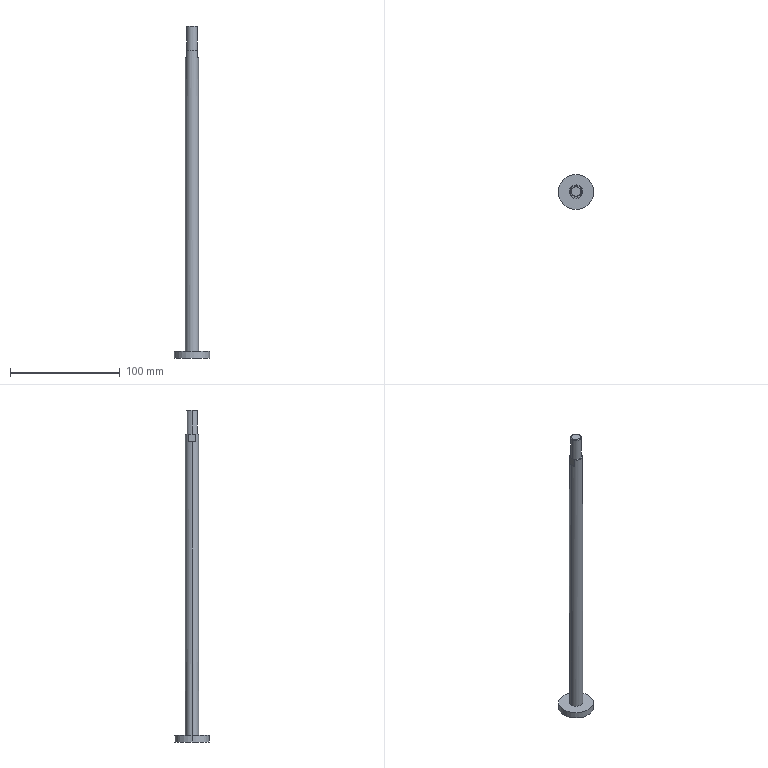Part | STEP file | 1 solid | 17 faces | box 32 x 32 x 303.2 mm | volume 37606 mm3 | plane 9 | cylinder 6 | cone 2 | commonest cylinder face diameters 10 x2 12 x2 32 x2
STEP:
#1=CARTESIAN_POINT('',(0.,0.,0.));
#2=DIRECTION('',(0.,0.,1.));
#3=DIRECTION('',(1.,0.,0.));
#4=AXIS2_PLACEMENT_3D('',#1,#2,#3);
#5=CARTESIAN_POINT('',(5.,0.,26.));
#6=VERTEX_POINT('',#5);
#7=CARTESIAN_POINT('',(-5.,0.,26.));
#8=VERTEX_POINT('',#7);
#9=CARTESIAN_POINT('',(0.,0.,26.));
#10=DIRECTION('',(0.,0.,1.));
#11=DIRECTION('',(1.,0.,0.));
#12=AXIS2_PLACEMENT_3D('',#9,#10,#11);
#13=CIRCLE('',#12,5.);
#14=CARTESIAN_POINT('',(0.,0.,26.));
#15=DIRECTION('',(0.,0.,1.));
#16=DIRECTION('',(1.,0.,0.));
#17=AXIS2_PLACEMENT_3D('',#14,#15,#16);
#18=CYLINDRICAL_SURFACE('',#17,5.);
#19=CARTESIAN_POINT('',(0.,0.));
#20=DIRECTION('',(1.,0.));
#21=VECTOR('',#20,1.);
#22=LINE('',#19,#21);
#23=(GEOMETRIC_REPRESENTATION_CONTEXT(2)PARAMETRIC_REPRESENTATION_CONTEXT()REPRESENTATION_CONTEXT('',''));
#24=DEFINITIONAL_REPRESENTATION('',(#22),#23);
#25=PCURVE('',#18,#24);
#26=CARTESIAN_POINT('',(0.,0.,26.));
#27=DIRECTION('',(0.,0.,-1.));
#28=DIRECTION('',(-1.,0.,0.));
#29=AXIS2_PLACEMENT_3D('',#26,#27,#28);
#30=PLANE('',#29);
#31=CARTESIAN_POINT('',(-5.,0.));
#32=CARTESIAN_POINT('',(-5.,8.66));
#33=CARTESIAN_POINT('',(2.5,4.33));
#34=CARTESIAN_POINT('',(10.,0.));
#35=CARTESIAN_POINT('',(2.5,-4.33));
#36=CARTESIAN_POINT('',(-5.,-8.66));
#37=CARTESIAN_POINT('',(-5.,0.));
#38=(BOUNDED_CURVE()B_SPLINE_CURVE(2,(#31,#32,#33,#34,#35,#36,#37),.UNSPECIFIED.,.T.,.F.)B_SPLINE_CURVE_WITH_KNOTS((1,2,2,2,2,1),(-2.094,0.,2.094,4.189,6.283,8.378),.UNSPECIFIED.)CURVE()GEOMETRIC_REPRESENTATION_ITEM()RATIONAL_B_SPLINE_CURVE((1.,0.5,1.,0.5,1.,0.5,1.))REPRESENTATION_ITEM(''));
#39=(GEOMETRIC_REPRESENTATION_CONTEXT(2)PARAMETRIC_REPRESENTATION_CONTEXT()REPRESENTATION_CONTEXT('',''));
#40=DEFINITIONAL_REPRESENTATION('',(#38),#39);
#41=PCURVE('',#30,#40);
#42=SURFACE_CURVE('',#13,(#25,#41),.PCURVE_S1.);
#43=EDGE_CURVE('',#6,#8,#42,.T.);
#44=ORIENTED_EDGE('',*,*,#43,.T.);
#45=CARTESIAN_POINT('',(-5.,0.,47.233));
#46=VERTEX_POINT('',#45);
#47=CARTESIAN_POINT('',(-5.,0.,26.));
#48=DIRECTION('',(0.,0.,1.));
#49=VECTOR('',#48,1.);
#50=LINE('',#47,#49);
#51=CARTESIAN_POINT('',(3.142,0.));
#52=DIRECTION('',(0.,1.));
#53=VECTOR('',#52,1.);
#54=LINE('',#51,#53);
#55=(GEOMETRIC_REPRESENTATION_CONTEXT(2)PARAMETRIC_REPRESENTATION_CONTEXT()REPRESENTATION_CONTEXT('',''));
#56=DEFINITIONAL_REPRESENTATION('',(#54),#55);
#57=PCURVE('',#18,#56);
#58=CARTESIAN_POINT('',(0.,0.,26.));
#59=DIRECTION('',(0.,0.,1.));
#60=DIRECTION('',(1.,0.,0.));
#61=AXIS2_PLACEMENT_3D('',#58,#59,#60);
#62=CYLINDRICAL_SURFACE('',#61,5.);
#63=CARTESIAN_POINT('',(3.142,0.));
#64=DIRECTION('',(0.,1.));
#65=VECTOR('',#64,1.);
#66=LINE('',#63,#65);
#67=(GEOMETRIC_REPRESENTATION_CONTEXT(2)PARAMETRIC_REPRESENTATION_CONTEXT()REPRESENTATION_CONTEXT('',''));
#68=DEFINITIONAL_REPRESENTATION('',(#66),#67);
#69=PCURVE('',#62,#68);
#70=SURFACE_CURVE('',#50,(#57,#69),.PCURVE_S1.);
#71=EDGE_CURVE('',#8,#46,#70,.T.);
#72=ORIENTED_EDGE('',*,*,#71,.T.);
#73=CARTESIAN_POINT('',(5.,0.,47.233));
#74=VERTEX_POINT('',#73);
#75=CARTESIAN_POINT('',(0.,0.,47.233));
#76=DIRECTION('',(0.,0.,1.));
#77=DIRECTION('',(1.,0.,0.));
#78=AXIS2_PLACEMENT_3D('',#75,#76,#77);
#79=CIRCLE('',#78,5.);
#80=CARTESIAN_POINT('',(0.,21.233));
#81=DIRECTION('',(1.,0.));
#82=VECTOR('',#81,1.);
#83=LINE('',#80,#82);
#84=(GEOMETRIC_REPRESENTATION_CONTEXT(2)PARAMETRIC_REPRESENTATION_CONTEXT()REPRESENTATION_CONTEXT('',''));
#85=DEFINITIONAL_REPRESENTATION('',(#83),#84);
#86=PCURVE('',#18,#85);
#87=CARTESIAN_POINT('',(0.,0.,47.233));
#88=DIRECTION('',(0.,0.,-1.));
#89=DIRECTION('',(-1.,0.,0.));
#90=AXIS2_PLACEMENT_3D('',#87,#88,#89);
#91=CONICAL_SURFACE('',#90,5.,0.7854);
#92=CARTESIAN_POINT('',(3.142,0.));
#93=DIRECTION('',(-1.,0.));
#94=VECTOR('',#93,1.);
#95=LINE('',#92,#94);
#96=(GEOMETRIC_REPRESENTATION_CONTEXT(2)PARAMETRIC_REPRESENTATION_CONTEXT()REPRESENTATION_CONTEXT('',''));
#97=DEFINITIONAL_REPRESENTATION('',(#95),#96);
#98=PCURVE('',#91,#97);
#99=SURFACE_CURVE('',#79,(#86,#98),.PCURVE_S1.);
#100=EDGE_CURVE('',#74,#46,#99,.T.);
#101=ORIENTED_EDGE('',*,*,#100,.F.);
#102=CARTESIAN_POINT('',(5.,0.,26.));
#103=DIRECTION('',(0.,0.,1.));
#104=VECTOR('',#103,1.);
#105=LINE('',#102,#104);
#106=CARTESIAN_POINT('',(0.,0.));
#107=DIRECTION('',(0.,1.));
#108=VECTOR('',#107,1.);
#109=LINE('',#106,#108);
#110=(GEOMETRIC_REPRESENTATION_CONTEXT(2)PARAMETRIC_REPRESENTATION_CONTEXT()REPRESENTATION_CONTEXT('',''));
#111=DEFINITIONAL_REPRESENTATION('',(#109),#110);
#112=PCURVE('',#18,#111);
#113=CARTESIAN_POINT('',(6.283,0.));
#114=DIRECTION('',(0.,1.));
#115=VECTOR('',#114,1.);
#116=LINE('',#113,#115);
#117=(GEOMETRIC_REPRESENTATION_CONTEXT(2)PARAMETRIC_REPRESENTATION_CONTEXT()REPRESENTATION_CONTEXT('',''));
#118=DEFINITIONAL_REPRESENTATION('',(#116),#117);
#119=PCURVE('',#62,#118);
#120=SURFACE_CURVE('',#105,(#112,#119),.PCURVE_S1.);
#121=EDGE_CURVE('',#6,#74,#120,.T.);
#122=ORIENTED_EDGE('',*,*,#121,.F.);
#123=EDGE_LOOP('',(#44,#72,#101,#122));
#124=FACE_BOUND('',#123,.T.);
#125=ADVANCED_FACE('',(#124),#18,.T.);
#126=CARTESIAN_POINT('',(4.233,0.,48.));
#127=VERTEX_POINT('',#126);
#128=CARTESIAN_POINT('',(-4.233,0.,48.));
#129=VERTEX_POINT('',#128);
#130=CARTESIAN_POINT('',(0.,0.,48.));
#131=DIRECTION('',(0.,0.,1.));
#132=DIRECTION('',(1.,0.,0.));
#133=AXIS2_PLACEMENT_3D('',#130,#131,#132);
#134=CIRCLE('',#133,4.233);
#135=CARTESIAN_POINT('',(3.142,-0.767));
#136=DIRECTION('',(-1.,0.));
#137=VECTOR('',#136,1.);
#138=LINE('',#135,#137);
#139=(GEOMETRIC_REPRESENTATION_CONTEXT(2)PARAMETRIC_REPRESENTATION_CONTEXT()REPRESENTATION_CONTEXT('',''));
#140=DEFINITIONAL_REPRESENTATION('',(#138),#139);
#141=PCURVE('',#91,#140);
#142=CARTESIAN_POINT('',(0.,0.,48.));
#143=DIRECTION('',(0.,0.,-1.));
#144=DIRECTION('',(-1.,0.,0.));
#145=AXIS2_PLACEMENT_3D('',#142,#143,#144);
#146=PLANE('',#145);
#147=CARTESIAN_POINT('',(-4.233,0.));
#148=CARTESIAN_POINT('',(-4.233,7.332));
#149=CARTESIAN_POINT('',(2.116,3.666));
#150=CARTESIAN_POINT('',(8.466,0.));
#151=CARTESIAN_POINT('',(2.116,-3.666));
#152=CARTESIAN_POINT('',(-4.233,-7.332));
#153=CARTESIAN_POINT('',(-4.233,0.));
#154=(BOUNDED_CURVE()B_SPLINE_CURVE(2,(#147,#148,#149,#150,#151,#152,#153),.UNSPECIFIED.,.T.,.F.)B_SPLINE_CURVE_WITH_KNOTS((1,2,2,2,2,1),(-2.094,0.,2.094,4.189,6.283,8.378),.UNSPECIFIED.)CURVE()GEOMETRIC_REPRESENTATION_ITEM()RATIONAL_B_SPLINE_CURVE((1.,0.5,1.,0.5,1.,0.5,1.))REPRESENTATION_ITEM(''));
#155=(GEOMETRIC_REPRESENTATION_CONTEXT(2)PARAMETRIC_REPRESENTATION_CONTEXT()REPRESENTATION_CONTEXT('',''));
#156=DEFINITIONAL_REPRESENTATION('',(#154),#155);
#157=PCURVE('',#146,#156);
#158=SURFACE_CURVE('',#134,(#141,#157),.PCURVE_S1.);
#159=EDGE_CURVE('',#127,#129,#158,.T.);
#160=ORIENTED_EDGE('',*,*,#159,.F.);
#161=CARTESIAN_POINT('',(5.,0.,47.233));
#162=DIRECTION('',(0.7071,0.,-0.7071));
#163=VECTOR('',#162,1.);
#164=LINE('',#161,#163);
#165=CARTESIAN_POINT('',(3.142,0.));
#166=DIRECTION('',(0.,1.));
#167=VECTOR('',#166,1.);
#168=LINE('',#165,#167);
#169=(GEOMETRIC_REPRESENTATION_CONTEXT(2)PARAMETRIC_REPRESENTATION_CONTEXT()REPRESENTATION_CONTEXT('',''));
#170=DEFINITIONAL_REPRESENTATION('',(#168),#169);
#171=PCURVE('',#91,#170);
#172=CARTESIAN_POINT('',(0.,0.,47.233));
#173=DIRECTION('',(0.,0.,-1.));
#174=DIRECTION('',(-1.,0.,0.));
#175=AXIS2_PLACEMENT_3D('',#172,#173,#174);
#176=CONICAL_SURFACE('',#175,5.,0.7854);
#177=CARTESIAN_POINT('',(3.142,0.));
#178=DIRECTION('',(0.,1.));
#179=VECTOR('',#178,1.);
#180=LINE('',#177,#179);
#181=(GEOMETRIC_REPRESENTATION_CONTEXT(2)PARAMETRIC_REPRESENTATION_CONTEXT()REPRESENTATION_CONTEXT('',''));
#182=DEFINITIONAL_REPRESENTATION('',(#180),#181);
#183=PCURVE('',#176,#182);
#184=SURFACE_CURVE('',#164,(#171,#183),.PCURVE_S1.);
#185=EDGE_CURVE('',#127,#74,#184,.T.);
#186=ORIENTED_EDGE('',*,*,#185,.T.);
#187=ORIENTED_EDGE('',*,*,#100,.T.);
#188=CARTESIAN_POINT('',(-5.,0.,47.233));
#189=DIRECTION('',(-0.7071,0.,-0.7071));
#190=VECTOR('',#189,1.);
#191=LINE('',#188,#190);
#192=CARTESIAN_POINT('',(0.,0.));
#193=DIRECTION('',(0.,1.));
#194=VECTOR('',#193,1.);
#195=LINE('',#192,#194);
#196=(GEOMETRIC_REPRESENTATION_CONTEXT(2)PARAMETRIC_REPRESENTATION_CONTEXT()REPRESENTATION_CONTEXT('',''));
#197=DEFINITIONAL_REPRESENTATION('',(#195),#196);
#198=PCURVE('',#91,#197);
#199=CARTESIAN_POINT('',(6.283,0.));
#200=DIRECTION('',(0.,1.));
#201=VECTOR('',#200,1.);
#202=LINE('',#199,#201);
#203=(GEOMETRIC_REPRESENTATION_CONTEXT(2)PARAMETRIC_REPRESENTATION_CONTEXT()REPRESENTATION_CONTEXT('',''));
#204=DEFINITIONAL_REPRESENTATION('',(#202),#203);
#205=PCURVE('',#176,#204);
#206=SURFACE_CURVE('',#191,(#198,#205),.PCURVE_S1.);
#207=EDGE_CURVE('',#129,#46,#206,.T.);
#208=ORIENTED_EDGE('',*,*,#207,.F.);
#209=EDGE_LOOP('',(#160,#186,#187,#208));
#210=FACE_BOUND('',#209,.T.);
#211=ADVANCED_FACE('',(#210),#91,.T.);
#212=CARTESIAN_POINT('',(16.,0.,-255.2));
#213=VERTEX_POINT('',#212);
#214=CARTESIAN_POINT('',(-16.,0.,-255.2));
#215=VERTEX_POINT('',#214);
#216=CARTESIAN_POINT('',(0.,0.,-255.2));
#217=DIRECTION('',(0.,0.,1.));
#218=DIRECTION('',(1.,0.,0.));
#219=AXIS2_PLACEMENT_3D('',#216,#217,#218);
#220=CIRCLE('',#219,16.);
#221=CARTESIAN_POINT('',(0.,0.,-255.2));
#222=DIRECTION('',(0.,0.,1.));
#223=DIRECTION('',(1.,0.,0.));
#224=AXIS2_PLACEMENT_3D('',#221,#222,#223);
#225=CYLINDRICAL_SURFACE('',#224,16.);
#226=CARTESIAN_POINT('',(0.,0.));
#227=DIRECTION('',(1.,0.));
#228=VECTOR('',#227,1.);
#229=LINE('',#226,#228);
#230=(GEOMETRIC_REPRESENTATION_CONTEXT(2)PARAMETRIC_REPRESENTATION_CONTEXT()REPRESENTATION_CONTEXT('',''));
#231=DEFINITIONAL_REPRESENTATION('',(#229),#230);
#232=PCURVE('',#225,#231);
#233=CARTESIAN_POINT('',(0.,16.,-255.2));
#234=DIRECTION('',(0.,0.,1.));
#235=DIRECTION('',(1.,0.,0.));
#236=AXIS2_PLACEMENT_3D('',#233,#234,#235);
#237=PLANE('',#236);
#238=CARTESIAN_POINT('',(0.,-16.));
#239=DIRECTION('',(1.,0.));
#240=AXIS2_PLACEMENT_2D('',#238,#239);
#241=CIRCLE('',#240,16.);
#242=(GEOMETRIC_REPRESENTATION_CONTEXT(2)PARAMETRIC_REPRESENTATION_CONTEXT()REPRESENTATION_CONTEXT('',''));
#243=DEFINITIONAL_REPRESENTATION('',(#241),#242);
#244=PCURVE('',#237,#243);
#245=SURFACE_CURVE('',#220,(#232,#244),.PCURVE_S1.);
#246=EDGE_CURVE('',#213,#215,#245,.T.);
#247=ORIENTED_EDGE('',*,*,#246,.T.);
#248=CARTESIAN_POINT('',(-16.,0.,-249.2));
#249=VERTEX_POINT('',#248);
#250=CARTESIAN_POINT('',(-16.,0.,-255.2));
#251=DIRECTION('',(0.,0.,1.));
#252=VECTOR('',#251,1.);
#253=LINE('',#250,#252);
#254=CARTESIAN_POINT('',(3.142,0.));
#255=DIRECTION('',(0.,1.));
#256=VECTOR('',#255,1.);
#257=LINE('',#254,#256);
#258=(GEOMETRIC_REPRESENTATION_CONTEXT(2)PARAMETRIC_REPRESENTATION_CONTEXT()REPRESENTATION_CONTEXT('',''));
#259=DEFINITIONAL_REPRESENTATION('',(#257),#258);
#260=PCURVE('',#225,#259);
#261=CARTESIAN_POINT('',(0.,0.,-255.2));
#262=DIRECTION('',(0.,0.,1.));
#263=DIRECTION('',(1.,0.,0.));
#264=AXIS2_PLACEMENT_3D('',#261,#262,#263);
#265=CYLINDRICAL_SURFACE('',#264,16.);
#266=CARTESIAN_POINT('',(3.142,0.));
#267=DIRECTION('',(0.,1.));
#268=VECTOR('',#267,1.);
#269=LINE('',#266,#268);
#270=(GEOMETRIC_REPRESENTATION_CONTEXT(2)PARAMETRIC_REPRESENTATION_CONTEXT()REPRESENTATION_CONTEXT('',''));
#271=DEFINITIONAL_REPRESENTATION('',(#269),#270);
#272=PCURVE('',#265,#271);
#273=SURFACE_CURVE('',#253,(#260,#272),.PCURVE_S1.);
#274=EDGE_CURVE('',#215,#249,#273,.T.);
#275=ORIENTED_EDGE('',*,*,#274,.T.);
#276=CARTESIAN_POINT('',(16.,0.,-249.2));
#277=VERTEX_POINT('',#276);
#278=CARTESIAN_POINT('',(0.,0.,-249.2));
#279=DIRECTION('',(0.,0.,1.));
#280=DIRECTION('',(1.,0.,0.));
#281=AXIS2_PLACEMENT_3D('',#278,#279,#280);
#282=CIRCLE('',#281,16.);
#283=CARTESIAN_POINT('',(0.,6.));
#284=DIRECTION('',(1.,0.));
#285=VECTOR('',#284,1.);
#286=LINE('',#283,#285);
#287=(GEOMETRIC_REPRESENTATION_CONTEXT(2)PARAMETRIC_REPRESENTATION_CONTEXT()REPRESENTATION_CONTEXT('',''));
#288=DEFINITIONAL_REPRESENTATION('',(#286),#287);
#289=PCURVE('',#225,#288);
#290=CARTESIAN_POINT('',(0.,6.,-249.2));
#291=DIRECTION('',(0.,0.,-1.));
#292=DIRECTION('',(-1.,0.,0.));
#293=AXIS2_PLACEMENT_3D('',#290,#291,#292);
#294=PLANE('',#293);
#295=CARTESIAN_POINT('',(-16.,-6.));
#296=CARTESIAN_POINT('',(-16.,21.713));
#297=CARTESIAN_POINT('',(8.,7.856));
#298=CARTESIAN_POINT('',(32.,-6.));
#299=CARTESIAN_POINT('',(8.,-19.856));
#300=CARTESIAN_POINT('',(-16.,-33.713));
#301=CARTESIAN_POINT('',(-16.,-6.));
#302=(BOUNDED_CURVE()B_SPLINE_CURVE(2,(#295,#296,#297,#298,#299,#300,#301),.UNSPECIFIED.,.T.,.F.)B_SPLINE_CURVE_WITH_KNOTS((1,2,2,2,2,1),(-2.094,0.,2.094,4.189,6.283,8.378),.UNSPECIFIED.)CURVE()GEOMETRIC_REPRESENTATION_ITEM()RATIONAL_B_SPLINE_CURVE((1.,0.5,1.,0.5,1.,0.5,1.))REPRESENTATION_ITEM(''));
#303=(GEOMETRIC_REPRESENTATION_CONTEXT(2)PARAMETRIC_REPRESENTATION_CONTEXT()REPRESENTATION_CONTEXT('',''));
#304=DEFINITIONAL_REPRESENTATION('',(#302),#303);
#305=PCURVE('',#294,#304);
#306=SURFACE_CURVE('',#282,(#289,#305),.PCURVE_S1.);
#307=EDGE_CURVE('',#277,#249,#306,.T.);
#308=ORIENTED_EDGE('',*,*,#307,.F.);
#309=CARTESIAN_POINT('',(16.,0.,-255.2));
#310=DIRECTION('',(0.,0.,1.));
#311=VECTOR('',#310,1.);
#312=LINE('',#309,#311);
#313=CARTESIAN_POINT('',(0.,0.));
#314=DIRECTION('',(0.,1.));
#315=VECTOR('',#314,1.);
#316=LINE('',#313,#315);
#317=(GEOMETRIC_REPRESENTATION_CONTEXT(2)PARAMETRIC_REPRESENTATION_CONTEXT()REPRESENTATION_CONTEXT('',''));
#318=DEFINITIONAL_REPRESENTATION('',(#316),#317);
#319=PCURVE('',#225,#318);
#320=CARTESIAN_POINT('',(6.283,0.));
#321=DIRECTION('',(0.,1.));
#322=VECTOR('',#321,1.);
#323=LINE('',#320,#322);
#324=(GEOMETRIC_REPRESENTATION_CONTEXT(2)PARAMETRIC_REPRESENTATION_CONTEXT()REPRESENTATION_CONTEXT('',''));
#325=DEFINITIONAL_REPRESENTATION('',(#323),#324);
#326=PCURVE('',#265,#325);
#327=SURFACE_CURVE('',#312,(#319,#326),.PCURVE_S1.);
#328=EDGE_CURVE('',#213,#277,#327,.T.);
#329=ORIENTED_EDGE('',*,*,#328,.F.);
#330=EDGE_LOOP('',(#247,#275,#308,#329));
#331=FACE_BOUND('',#330,.T.);
#332=ADVANCED_FACE('',(#331),#225,.T.);
#333=CARTESIAN_POINT('',(6.,0.,-249.2));
#334=VERTEX_POINT('',#333);
#335=CARTESIAN_POINT('',(-6.,0.,-249.2));
#336=VERTEX_POINT('',#335);
#337=CARTESIAN_POINT('',(0.,0.,-249.2));
#338=DIRECTION('',(0.,0.,1.));
#339=DIRECTION('',(1.,0.,0.));
#340=AXIS2_PLACEMENT_3D('',#337,#338,#339);
#341=CIRCLE('',#340,6.);
#342=CARTESIAN_POINT('',(0.,0.,-255.2));
#343=DIRECTION('',(0.,0.,1.));
#344=DIRECTION('',(1.,0.,0.));
#345=AXIS2_PLACEMENT_3D('',#342,#343,#344);
#346=CYLINDRICAL_SURFACE('',#345,6.);
#347=CARTESIAN_POINT('',(0.,6.));
#348=DIRECTION('',(1.,0.));
#349=VECTOR('',#348,1.);
#350=LINE('',#347,#349);
#351=(GEOMETRIC_REPRESENTATION_CONTEXT(2)PARAMETRIC_REPRESENTATION_CONTEXT()REPRESENTATION_CONTEXT('',''));
#352=DEFINITIONAL_REPRESENTATION('',(#350),#351);
#353=PCURVE('',#346,#352);
#354=CARTESIAN_POINT('',(-6.,-6.));
#355=CARTESIAN_POINT('',(-6.,4.392));
#356=CARTESIAN_POINT('',(3.,-0.8038));
#357=CARTESIAN_POINT('',(12.,-6.));
#358=CARTESIAN_POINT('',(3.,-11.196));
#359=CARTESIAN_POINT('',(-6.,-16.392));
#360=CARTESIAN_POINT('',(-6.,-6.));
#361=(BOUNDED_CURVE()B_SPLINE_CURVE(2,(#354,#355,#356,#357,#358,#359,#360),.UNSPECIFIED.,.T.,.F.)B_SPLINE_CURVE_WITH_KNOTS((1,2,2,2,2,1),(-2.094,0.,2.094,4.189,6.283,8.378),.UNSPECIFIED.)CURVE()GEOMETRIC_REPRESENTATION_ITEM()RATIONAL_B_SPLINE_CURVE((1.,0.5,1.,0.5,1.,0.5,1.))REPRESENTATION_ITEM(''));
#362=(GEOMETRIC_REPRESENTATION_CONTEXT(2)PARAMETRIC_REPRESENTATION_CONTEXT()REPRESENTATION_CONTEXT('',''));
#363=DEFINITIONAL_REPRESENTATION('',(#361),#362);
#364=PCURVE('',#294,#363);
#365=SURFACE_CURVE('',#341,(#353,#364),.PCURVE_S1.);
#366=EDGE_CURVE('',#334,#336,#365,.T.);
#367=ORIENTED_EDGE('',*,*,#366,.T.);
#368=CARTESIAN_POINT('',(-6.,0.,19.));
#369=VERTEX_POINT('',#368);
#370=CARTESIAN_POINT('',(-6.,0.,-255.2));
#371=DIRECTION('',(0.,0.,1.));
#372=VECTOR('',#371,1.);
#373=LINE('',#370,#372);
#374=CARTESIAN_POINT('',(3.142,0.));
#375=DIRECTION('',(0.,1.));
#376=VECTOR('',#375,1.);
#377=LINE('',#374,#376);
#378=(GEOMETRIC_REPRESENTATION_CONTEXT(2)PARAMETRIC_REPRESENTATION_CONTEXT()REPRESENTATION_CONTEXT('',''));
#379=DEFINITIONAL_REPRESENTATION('',(#377),#378);
#380=PCURVE('',#346,#379);
#381=CARTESIAN_POINT('',(0.,0.,-255.2));
#382=DIRECTION('',(0.,0.,1.));
#383=DIRECTION('',(1.,0.,0.));
#384=AXIS2_PLACEMENT_3D('',#381,#382,#383);
#385=CYLINDRICAL_SURFACE('',#384,6.);
#386=CARTESIAN_POINT('',(3.142,0.));
#387=DIRECTION('',(0.,1.));
#388=VECTOR('',#387,1.);
#389=LINE('',#386,#388);
#390=(GEOMETRIC_REPRESENTATION_CONTEXT(2)PARAMETRIC_REPRESENTATION_CONTEXT()REPRESENTATION_CONTEXT('',''));
#391=DEFINITIONAL_REPRESENTATION('',(#389),#390);
#392=PCURVE('',#385,#391);
#393=SURFACE_CURVE('',#373,(#380,#392),.PCURVE_S1.);
#394=EDGE_CURVE('',#336,#369,#393,.T.);
#395=ORIENTED_EDGE('',*,*,#394,.T.);
#396=CARTESIAN_POINT('',(-5.,3.317,19.));
#397=VERTEX_POINT('',#396);
#398=CARTESIAN_POINT('',(0.,0.,19.));
#399=DIRECTION('',(0.,0.,1.));
#400=DIRECTION('',(1.,0.,0.));
#401=AXIS2_PLACEMENT_3D('',#398,#399,#400);
#402=CIRCLE('',#401,6.);
#403=CARTESIAN_POINT('',(0.,274.2));
#404=DIRECTION('',(1.,0.));
#405=VECTOR('',#404,1.);
#406=LINE('',#403,#405);
#407=(GEOMETRIC_REPRESENTATION_CONTEXT(2)PARAMETRIC_REPRESENTATION_CONTEXT()REPRESENTATION_CONTEXT('',''));
#408=DEFINITIONAL_REPRESENTATION('',(#406),#407);
#409=PCURVE('',#346,#408);
#410=CARTESIAN_POINT('',(0.,0.,19.));
#411=DIRECTION('',(0.,0.,1.));
#412=DIRECTION('',(1.,0.,0.));
#413=AXIS2_PLACEMENT_3D('',#410,#411,#412);
#414=PLANE('',#413);
#415=CARTESIAN_POINT('',(0.,0.));
#416=DIRECTION('',(1.,0.));
#417=AXIS2_PLACEMENT_2D('',#415,#416);
#418=CIRCLE('',#417,6.);
#419=(GEOMETRIC_REPRESENTATION_CONTEXT(2)PARAMETRIC_REPRESENTATION_CONTEXT()REPRESENTATION_CONTEXT('',''));
#420=DEFINITIONAL_REPRESENTATION('',(#418),#419);
#421=PCURVE('',#414,#420);
#422=SURFACE_CURVE('',#402,(#409,#421),.PCURVE_S1.);
#423=EDGE_CURVE('',#397,#369,#422,.T.);
#424=ORIENTED_EDGE('',*,*,#423,.F.);
#425=CARTESIAN_POINT('',(-5.,3.317,26.));
#426=VERTEX_POINT('',#425);
#427=CARTESIAN_POINT('',(-5.,3.317,-255.2));
#428=DIRECTION('',(0.,0.,1.));
#429=VECTOR('',#428,1.);
#430=LINE('',#427,#429);
#431=CARTESIAN_POINT('',(2.556,0.));
#432=DIRECTION('',(0.,1.));
#433=VECTOR('',#432,1.);
#434=LINE('',#431,#433);
#435=(GEOMETRIC_REPRESENTATION_CONTEXT(2)PARAMETRIC_REPRESENTATION_CONTEXT()REPRESENTATION_CONTEXT('',''));
#436=DEFINITIONAL_REPRESENTATION('',(#434),#435);
#437=PCURVE('',#346,#436);
#438=CARTESIAN_POINT('',(-5.,-10.,19.));
#439=DIRECTION('',(1.,0.,0.));
#440=DIRECTION('',(0.,0.,-1.));
#441=AXIS2_PLACEMENT_3D('',#438,#439,#440);
#442=PLANE('',#441);
#443=CARTESIAN_POINT('',(274.2,13.317));
#444=DIRECTION('',(-1.,0.));
#445=VECTOR('',#444,1.);
#446=LINE('',#443,#445);
#447=(GEOMETRIC_REPRESENTATION_CONTEXT(2)PARAMETRIC_REPRESENTATION_CONTEXT()REPRESENTATION_CONTEXT('',''));
#448=DEFINITIONAL_REPRESENTATION('',(#446),#447);
#449=PCURVE('',#442,#448);
#450=SURFACE_CURVE('',#430,(#437,#449),.PCURVE_S1.);
#451=EDGE_CURVE('',#397,#426,#450,.T.);
#452=ORIENTED_EDGE('',*,*,#451,.T.);
#453=CARTESIAN_POINT('',(5.,3.317,26.));
#454=VERTEX_POINT('',#453);
#455=CARTESIAN_POINT('',(0.,0.,26.));
#456=DIRECTION('',(0.,0.,1.));
#457=DIRECTION('',(1.,0.,0.));
#458=AXIS2_PLACEMENT_3D('',#455,#456,#457);
#459=CIRCLE('',#458,6.);
#460=CARTESIAN_POINT('',(0.,281.2));
#461=DIRECTION('',(1.,0.));
#462=VECTOR('',#461,1.);
#463=LINE('',#460,#462);
#464=(GEOMETRIC_REPRESENTATION_CONTEXT(2)PARAMETRIC_REPRESENTATION_CONTEXT()REPRESENTATION_CONTEXT('',''));
#465=DEFINITIONAL_REPRESENTATION('',(#463),#464);
#466=PCURVE('',#346,#465);
#467=CARTESIAN_POINT('',(-6.,0.));
#468=CARTESIAN_POINT('',(-6.,10.392));
#469=CARTESIAN_POINT('',(3.,5.196));
#470=CARTESIAN_POINT('',(12.,0.));
#471=CARTESIAN_POINT('',(3.,-5.196));
#472=CARTESIAN_POINT('',(-6.,-10.392));
#473=CARTESIAN_POINT('',(-6.,0.));
#474=(BOUNDED_CURVE()B_SPLINE_CURVE(2,(#467,#468,#469,#470,#471,#472,#473),.UNSPECIFIED.,.T.,.F.)B_SPLINE_CURVE_WITH_KNOTS((1,2,2,2,2,1),(-2.094,0.,2.094,4.189,6.283,8.378),.UNSPECIFIED.)CURVE()GEOMETRIC_REPRESENTATION_ITEM()RATIONAL_B_SPLINE_CURVE((1.,0.5,1.,0.5,1.,0.5,1.))REPRESENTATION_ITEM(''));
#475=(GEOMETRIC_REPRESENTATION_CONTEXT(2)PARAMETRIC_REPRESENTATION_CONTEXT()REPRESENTATION_CONTEXT('',''));
#476=DEFINITIONAL_REPRESENTATION('',(#474),#475);
#477=PCURVE('',#30,#476);
#478=SURFACE_CURVE('',#459,(#466,#477),.PCURVE_S1.);
#479=EDGE_CURVE('',#454,#426,#478,.T.);
#480=ORIENTED_EDGE('',*,*,#479,.F.);
#481=CARTESIAN_POINT('',(5.,3.317,19.));
#482=VERTEX_POINT('',#481);
#483=CARTESIAN_POINT('',(5.,3.317,-255.2));
#484=DIRECTION('',(0.,0.,-1.));
#485=VECTOR('',#484,1.);
#486=LINE('',#483,#485);
#487=CARTESIAN_POINT('',(0.5857,0.));
#488=DIRECTION('',(0.,-1.));
#489=VECTOR('',#488,1.);
#490=LINE('',#487,#489);
#491=(GEOMETRIC_REPRESENTATION_CONTEXT(2)PARAMETRIC_REPRESENTATION_CONTEXT()REPRESENTATION_CONTEXT('',''));
#492=DEFINITIONAL_REPRESENTATION('',(#490),#491);
#493=PCURVE('',#346,#492);
#494=CARTESIAN_POINT('',(5.,10.,19.));
#495=DIRECTION('',(-1.,0.,0.));
#496=DIRECTION('',(0.,0.,1.));
#497=AXIS2_PLACEMENT_3D('',#494,#495,#496);
#498=PLANE('',#497);
#499=CARTESIAN_POINT('',(-274.2,-6.683));
#500=DIRECTION('',(-1.,0.));
#501=VECTOR('',#500,1.);
#502=LINE('',#499,#501);
#503=(GEOMETRIC_REPRESENTATION_CONTEXT(2)PARAMETRIC_REPRESENTATION_CONTEXT()REPRESENTATION_CONTEXT('',''));
#504=DEFINITIONAL_REPRESENTATION('',(#502),#503);
#505=PCURVE('',#498,#504);
#506=SURFACE_CURVE('',#486,(#493,#505),.PCURVE_S1.);
#507=EDGE_CURVE('',#454,#482,#506,.T.);
#508=ORIENTED_EDGE('',*,*,#507,.T.);
#509=CARTESIAN_POINT('',(6.,0.,19.));
#510=VERTEX_POINT('',#509);
#511=CARTESIAN_POINT('',(0.,0.,19.));
#512=DIRECTION('',(0.,0.,1.));
#513=DIRECTION('',(1.,0.,0.));
#514=AXIS2_PLACEMENT_3D('',#511,#512,#513);
#515=CIRCLE('',#514,6.);
#516=CARTESIAN_POINT('',(0.,274.2));
#517=DIRECTION('',(1.,0.));
#518=VECTOR('',#517,1.);
#519=LINE('',#516,#518);
#520=(GEOMETRIC_REPRESENTATION_CONTEXT(2)PARAMETRIC_REPRESENTATION_CONTEXT()REPRESENTATION_CONTEXT('',''));
#521=DEFINITIONAL_REPRESENTATION('',(#519),#520);
#522=PCURVE('',#346,#521);
#523=CARTESIAN_POINT('',(0.,0.,19.));
#524=DIRECTION('',(0.,0.,1.));
#525=DIRECTION('',(1.,0.,0.));
#526=AXIS2_PLACEMENT_3D('',#523,#524,#525);
#527=PLANE('',#526);
#528=CARTESIAN_POINT('',(0.,0.));
#529=DIRECTION('',(1.,0.));
#530=AXIS2_PLACEMENT_2D('',#528,#529);
#531=CIRCLE('',#530,6.);
#532=(GEOMETRIC_REPRESENTATION_CONTEXT(2)PARAMETRIC_REPRESENTATION_CONTEXT()REPRESENTATION_CONTEXT('',''));
#533=DEFINITIONAL_REPRESENTATION('',(#531),#532);
#534=PCURVE('',#527,#533);
#535=SURFACE_CURVE('',#515,(#522,#534),.PCURVE_S1.);
#536=EDGE_CURVE('',#510,#482,#535,.T.);
#537=ORIENTED_EDGE('',*,*,#536,.F.);
#538=CARTESIAN_POINT('',(6.,0.,-255.2));
#539=DIRECTION('',(0.,0.,1.));
#540=VECTOR('',#539,1.);
#541=LINE('',#538,#540);
#542=CARTESIAN_POINT('',(0.,0.));
#543=DIRECTION('',(0.,1.));
#544=VECTOR('',#543,1.);
#545=LINE('',#542,#544);
#546=(GEOMETRIC_REPRESENTATION_CONTEXT(2)PARAMETRIC_REPRESENTATION_CONTEXT()REPRESENTATION_CONTEXT('',''));
#547=DEFINITIONAL_REPRESENTATION('',(#545),#546);
#548=PCURVE('',#346,#547);
#549=CARTESIAN_POINT('',(6.283,0.));
#550=DIRECTION('',(0.,1.));
#551=VECTOR('',#550,1.);
#552=LINE('',#549,#551);
#553=(GEOMETRIC_REPRESENTATION_CONTEXT(2)PARAMETRIC_REPRESENTATION_CONTEXT()REPRESENTATION_CONTEXT('',''));
#554=DEFINITIONAL_REPRESENTATION('',(#552),#553);
#555=PCURVE('',#385,#554);
#556=SURFACE_CURVE('',#541,(#548,#555),.PCURVE_S1.);
#557=EDGE_CURVE('',#334,#510,#556,.T.);
#558=ORIENTED_EDGE('',*,*,#557,.F.);
#559=EDGE_LOOP('',(#367,#395,#424,#452,#480,#508,#537,#558));
#560=FACE_BOUND('',#559,.T.);
#561=ADVANCED_FACE('',(#560),#346,.T.);
#562=ORIENTED_EDGE('',*,*,#43,.F.);
#563=CARTESIAN_POINT('',(5.,10.,26.));
#564=DIRECTION('',(0.,-1.,0.));
#565=VECTOR('',#564,1.);
#566=LINE('',#563,#565);
#567=CARTESIAN_POINT('',(-5.,10.));
#568=DIRECTION('',(0.,-1.));
#569=VECTOR('',#568,1.);
#570=LINE('',#567,#569);
#571=(GEOMETRIC_REPRESENTATION_CONTEXT(2)PARAMETRIC_REPRESENTATION_CONTEXT()REPRESENTATION_CONTEXT('',''));
#572=DEFINITIONAL_REPRESENTATION('',(#570),#571);
#573=PCURVE('',#30,#572);
#574=CARTESIAN_POINT('',(7.,0.));
#575=DIRECTION('',(0.,-1.));
#576=VECTOR('',#575,1.);
#577=LINE('',#574,#576);
#578=(GEOMETRIC_REPRESENTATION_CONTEXT(2)PARAMETRIC_REPRESENTATION_CONTEXT()REPRESENTATION_CONTEXT('',''));
#579=DEFINITIONAL_REPRESENTATION('',(#577),#578);
#580=PCURVE('',#498,#579);
#581=SURFACE_CURVE('',#566,(#573,#580),.PCURVE_S1.);
#582=EDGE_CURVE('',#454,#6,#581,.T.);
#583=ORIENTED_EDGE('',*,*,#582,.F.);
#584=ORIENTED_EDGE('',*,*,#479,.T.);
#585=CARTESIAN_POINT('',(-5.,-10.,26.));
#586=DIRECTION('',(0.,1.,0.));
#587=VECTOR('',#586,1.);
#588=LINE('',#585,#587);
#589=CARTESIAN_POINT('',(5.,-10.));
#590=DIRECTION('',(0.,1.));
#591=VECTOR('',#590,1.);
#592=LINE('',#589,#591);
#593=(GEOMETRIC_REPRESENTATION_CONTEXT(2)PARAMETRIC_REPRESENTATION_CONTEXT()REPRESENTATION_CONTEXT('',''));
#594=DEFINITIONAL_REPRESENTATION('',(#592),#593);
#595=PCURVE('',#30,#594);
#596=CARTESIAN_POINT('',(-7.,0.));
#597=DIRECTION('',(0.,1.));
#598=VECTOR('',#597,1.);
#599=LINE('',#596,#598);
#600=(GEOMETRIC_REPRESENTATION_CONTEXT(2)PARAMETRIC_REPRESENTATION_CONTEXT()REPRESENTATION_CONTEXT('',''));
#601=DEFINITIONAL_REPRESENTATION('',(#599),#600);
#602=PCURVE('',#442,#601);
#603=SURFACE_CURVE('',#588,(#595,#602),.PCURVE_S1.);
#604=EDGE_CURVE('',#8,#426,#603,.T.);
#605=ORIENTED_EDGE('',*,*,#604,.F.);
#606=EDGE_LOOP('',(#562,#583,#584,#605));
#607=FACE_BOUND('',#606,.T.);
#608=ADVANCED_FACE('',(#607),#30,.F.);
#609=CARTESIAN_POINT('',(0.,0.,26.));
#610=DIRECTION('',(0.,0.,1.));
#611=DIRECTION('',(1.,0.,0.));
#612=AXIS2_PLACEMENT_3D('',#609,#610,#611);
#613=CIRCLE('',#612,5.);
#614=CARTESIAN_POINT('',(0.,0.,26.));
#615=DIRECTION('',(0.,0.,-1.));
#616=DIRECTION('',(-1.,0.,0.));
#617=AXIS2_PLACEMENT_3D('',#614,#615,#616);
#618=PLANE('',#617);
#619=CARTESIAN_POINT('',(-5.,0.));
#620=CARTESIAN_POINT('',(-5.,8.66));
#621=CARTESIAN_POINT('',(2.5,4.33));
#622=CARTESIAN_POINT('',(10.,0.));
#623=CARTESIAN_POINT('',(2.5,-4.33));
#624=CARTESIAN_POINT('',(-5.,-8.66));
#625=CARTESIAN_POINT('',(-5.,0.));
#626=(BOUNDED_CURVE()B_SPLINE_CURVE(2,(#619,#620,#621,#622,#623,#624,#625),.UNSPECIFIED.,.T.,.F.)B_SPLINE_CURVE_WITH_KNOTS((1,2,2,2,2,1),(-2.094,0.,2.094,4.189,6.283,8.378),.UNSPECIFIED.)CURVE()GEOMETRIC_REPRESENTATION_ITEM()RATIONAL_B_SPLINE_CURVE((1.,0.5,1.,0.5,1.,0.5,1.))REPRESENTATION_ITEM(''));
#627=(GEOMETRIC_REPRESENTATION_CONTEXT(2)PARAMETRIC_REPRESENTATION_CONTEXT()REPRESENTATION_CONTEXT('',''));
#628=DEFINITIONAL_REPRESENTATION('',(#626),#627);
#629=PCURVE('',#618,#628);
#630=CARTESIAN_POINT('',(0.,0.));
#631=DIRECTION('',(1.,0.));
#632=VECTOR('',#631,1.);
#633=LINE('',#630,#632);
#634=(GEOMETRIC_REPRESENTATION_CONTEXT(2)PARAMETRIC_REPRESENTATION_CONTEXT()REPRESENTATION_CONTEXT('',''));
#635=DEFINITIONAL_REPRESENTATION('',(#633),#634);
#636=PCURVE('',#62,#635);
#637=SURFACE_CURVE('',#613,(#629,#636),.PCURVE_S1.);
#638=EDGE_CURVE('',#8,#6,#637,.T.);
#639=ORIENTED_EDGE('',*,*,#638,.F.);
#640=CARTESIAN_POINT('',(-5.,-3.317,26.));
#641=VERTEX_POINT('',#640);
#642=CARTESIAN_POINT('',(-5.,-10.,26.));
#643=DIRECTION('',(0.,1.,0.));
#644=VECTOR('',#643,1.);
#645=LINE('',#642,#644);
#646=CARTESIAN_POINT('',(5.,-10.));
#647=DIRECTION('',(0.,1.));
#648=VECTOR('',#647,1.);
#649=LINE('',#646,#648);
#650=(GEOMETRIC_REPRESENTATION_CONTEXT(2)PARAMETRIC_REPRESENTATION_CONTEXT()REPRESENTATION_CONTEXT('',''));
#651=DEFINITIONAL_REPRESENTATION('',(#649),#650);
#652=PCURVE('',#618,#651);
#653=CARTESIAN_POINT('',(-7.,0.));
#654=DIRECTION('',(0.,1.));
#655=VECTOR('',#654,1.);
#656=LINE('',#653,#655);
#657=(GEOMETRIC_REPRESENTATION_CONTEXT(2)PARAMETRIC_REPRESENTATION_CONTEXT()REPRESENTATION_CONTEXT('',''));
#658=DEFINITIONAL_REPRESENTATION('',(#656),#657);
#659=PCURVE('',#442,#658);
#660=SURFACE_CURVE('',#645,(#652,#659),.PCURVE_S1.);
#661=EDGE_CURVE('',#641,#8,#660,.T.);
#662=ORIENTED_EDGE('',*,*,#661,.F.);
#663=CARTESIAN_POINT('',(5.,-3.317,26.));
#664=VERTEX_POINT('',#663);
#665=CARTESIAN_POINT('',(0.,0.,26.));
#666=DIRECTION('',(0.,0.,1.));
#667=DIRECTION('',(1.,0.,0.));
#668=AXIS2_PLACEMENT_3D('',#665,#666,#667);
#669=CIRCLE('',#668,6.);
#670=CARTESIAN_POINT('',(-6.,0.));
#671=CARTESIAN_POINT('',(-6.,10.392));
#672=CARTESIAN_POINT('',(3.,5.196));
#673=CARTESIAN_POINT('',(12.,0.));
#674=CARTESIAN_POINT('',(3.,-5.196));
#675=CARTESIAN_POINT('',(-6.,-10.392));
#676=CARTESIAN_POINT('',(-6.,0.));
#677=(BOUNDED_CURVE()B_SPLINE_CURVE(2,(#670,#671,#672,#673,#674,#675,#676),.UNSPECIFIED.,.T.,.F.)B_SPLINE_CURVE_WITH_KNOTS((1,2,2,2,2,1),(-2.094,0.,2.094,4.189,6.283,8.378),.UNSPECIFIED.)CURVE()GEOMETRIC_REPRESENTATION_ITEM()RATIONAL_B_SPLINE_CURVE((1.,0.5,1.,0.5,1.,0.5,1.))REPRESENTATION_ITEM(''));
#678=(GEOMETRIC_REPRESENTATION_CONTEXT(2)PARAMETRIC_REPRESENTATION_CONTEXT()REPRESENTATION_CONTEXT('',''));
#679=DEFINITIONAL_REPRESENTATION('',(#677),#678);
#680=PCURVE('',#618,#679);
#681=CARTESIAN_POINT('',(0.,281.2));
#682=DIRECTION('',(1.,0.));
#683=VECTOR('',#682,1.);
#684=LINE('',#681,#683);
#685=(GEOMETRIC_REPRESENTATION_CONTEXT(2)PARAMETRIC_REPRESENTATION_CONTEXT()REPRESENTATION_CONTEXT('',''));
#686=DEFINITIONAL_REPRESENTATION('',(#684),#685);
#687=PCURVE('',#385,#686);
#688=SURFACE_CURVE('',#669,(#680,#687),.PCURVE_S1.);
#689=EDGE_CURVE('',#641,#664,#688,.T.);
#690=ORIENTED_EDGE('',*,*,#689,.T.);
#691=CARTESIAN_POINT('',(5.,10.,26.));
#692=DIRECTION('',(0.,-1.,0.));
#693=VECTOR('',#692,1.);
#694=LINE('',#691,#693);
#695=CARTESIAN_POINT('',(-5.,10.));
#696=DIRECTION('',(0.,-1.));
#697=VECTOR('',#696,1.);
#698=LINE('',#695,#697);
#699=(GEOMETRIC_REPRESENTATION_CONTEXT(2)PARAMETRIC_REPRESENTATION_CONTEXT()REPRESENTATION_CONTEXT('',''));
#700=DEFINITIONAL_REPRESENTATION('',(#698),#699);
#701=PCURVE('',#618,#700);
#702=CARTESIAN_POINT('',(7.,0.));
#703=DIRECTION('',(0.,-1.));
#704=VECTOR('',#703,1.);
#705=LINE('',#702,#704);
#706=(GEOMETRIC_REPRESENTATION_CONTEXT(2)PARAMETRIC_REPRESENTATION_CONTEXT()REPRESENTATION_CONTEXT('',''));
#707=DEFINITIONAL_REPRESENTATION('',(#705),#706);
#708=PCURVE('',#498,#707);
#709=SURFACE_CURVE('',#694,(#701,#708),.PCURVE_S1.);
#710=EDGE_CURVE('',#6,#664,#709,.T.);
#711=ORIENTED_EDGE('',*,*,#710,.F.);
#712=EDGE_LOOP('',(#639,#662,#690,#711));
#713=FACE_BOUND('',#712,.T.);
#714=ADVANCED_FACE('',(#713),#618,.F.);
#715=ORIENTED_EDGE('',*,*,#394,.F.);
#716=CARTESIAN_POINT('',(0.,0.,-249.2));
#717=DIRECTION('',(0.,0.,1.));
#718=DIRECTION('',(1.,0.,0.));
#719=AXIS2_PLACEMENT_3D('',#716,#717,#718);
#720=CIRCLE('',#719,6.);
#721=CARTESIAN_POINT('',(0.,6.));
#722=DIRECTION('',(1.,0.));
#723=VECTOR('',#722,1.);
#724=LINE('',#721,#723);
#725=(GEOMETRIC_REPRESENTATION_CONTEXT(2)PARAMETRIC_REPRESENTATION_CONTEXT()REPRESENTATION_CONTEXT('',''));
#726=DEFINITIONAL_REPRESENTATION('',(#724),#725);
#727=PCURVE('',#385,#726);
#728=CARTESIAN_POINT('',(-6.,-6.));
#729=CARTESIAN_POINT('',(-6.,4.392));
#730=CARTESIAN_POINT('',(3.,-0.8038));
#731=CARTESIAN_POINT('',(12.,-6.));
#732=CARTESIAN_POINT('',(3.,-11.196));
#733=CARTESIAN_POINT('',(-6.,-16.392));
#734=CARTESIAN_POINT('',(-6.,-6.));
#735=(BOUNDED_CURVE()B_SPLINE_CURVE(2,(#728,#729,#730,#731,#732,#733,#734),.UNSPECIFIED.,.T.,.F.)B_SPLINE_CURVE_WITH_KNOTS((1,2,2,2,2,1),(-2.094,0.,2.094,4.189,6.283,8.378),.UNSPECIFIED.)CURVE()GEOMETRIC_REPRESENTATION_ITEM()RATIONAL_B_SPLINE_CURVE((1.,0.5,1.,0.5,1.,0.5,1.))REPRESENTATION_ITEM(''));
#736=(GEOMETRIC_REPRESENTATION_CONTEXT(2)PARAMETRIC_REPRESENTATION_CONTEXT()REPRESENTATION_CONTEXT('',''));
#737=DEFINITIONAL_REPRESENTATION('',(#735),#736);
#738=PCURVE('',#294,#737);
#739=SURFACE_CURVE('',#720,(#727,#738),.PCURVE_S1.);
#740=EDGE_CURVE('',#336,#334,#739,.T.);
#741=ORIENTED_EDGE('',*,*,#740,.T.);
#742=ORIENTED_EDGE('',*,*,#557,.T.);
#743=CARTESIAN_POINT('',(5.,-3.317,19.));
#744=VERTEX_POINT('',#743);
#745=CARTESIAN_POINT('',(0.,0.,19.));
#746=DIRECTION('',(0.,0.,1.));
#747=DIRECTION('',(1.,0.,0.));
#748=AXIS2_PLACEMENT_3D('',#745,#746,#747);
#749=CIRCLE('',#748,6.);
#750=CARTESIAN_POINT('',(0.,274.2));
#751=DIRECTION('',(1.,0.));
#752=VECTOR('',#751,1.);
#753=LINE('',#750,#752);
#754=(GEOMETRIC_REPRESENTATION_CONTEXT(2)PARAMETRIC_REPRESENTATION_CONTEXT()REPRESENTATION_CONTEXT('',''));
#755=DEFINITIONAL_REPRESENTATION('',(#753),#754);
#756=PCURVE('',#385,#755);
#757=CARTESIAN_POINT('',(0.,0.));
#758=DIRECTION('',(1.,0.));
#759=AXIS2_PLACEMENT_2D('',#757,#758);
#760=CIRCLE('',#759,6.);
#761=(GEOMETRIC_REPRESENTATION_CONTEXT(2)PARAMETRIC_REPRESENTATION_CONTEXT()REPRESENTATION_CONTEXT('',''));
#762=DEFINITIONAL_REPRESENTATION('',(#760),#761);
#763=PCURVE('',#527,#762);
#764=SURFACE_CURVE('',#749,(#756,#763),.PCURVE_S1.);
#765=EDGE_CURVE('',#744,#510,#764,.T.);
#766=ORIENTED_EDGE('',*,*,#765,.F.);
#767=CARTESIAN_POINT('',(5.,-3.317,-255.2));
#768=DIRECTION('',(0.,0.,1.));
#769=VECTOR('',#768,1.);
#770=LINE('',#767,#769);
#771=CARTESIAN_POINT('',(5.697,0.));
#772=DIRECTION('',(0.,1.));
#773=VECTOR('',#772,1.);
#774=LINE('',#771,#773);
#775=(GEOMETRIC_REPRESENTATION_CONTEXT(2)PARAMETRIC_REPRESENTATION_CONTEXT()REPRESENTATION_CONTEXT('',''));
#776=DEFINITIONAL_REPRESENTATION('',(#774),#775);
#777=PCURVE('',#385,#776);
#778=CARTESIAN_POINT('',(-274.2,-13.317));
#779=DIRECTION('',(1.,0.));
#780=VECTOR('',#779,1.);
#781=LINE('',#778,#780);
#782=(GEOMETRIC_REPRESENTATION_CONTEXT(2)PARAMETRIC_REPRESENTATION_CONTEXT()REPRESENTATION_CONTEXT('',''));
#783=DEFINITIONAL_REPRESENTATION('',(#781),#782);
#784=PCURVE('',#498,#783);
#785=SURFACE_CURVE('',#770,(#777,#784),.PCURVE_S1.);
#786=EDGE_CURVE('',#744,#664,#785,.T.);
#787=ORIENTED_EDGE('',*,*,#786,.T.);
#788=ORIENTED_EDGE('',*,*,#689,.F.);
#789=CARTESIAN_POINT('',(-5.,-3.317,19.));
#790=VERTEX_POINT('',#789);
#791=CARTESIAN_POINT('',(-5.,-3.317,-255.2));
#792=DIRECTION('',(0.,0.,-1.));
#793=VECTOR('',#792,1.);
#794=LINE('',#791,#793);
#795=CARTESIAN_POINT('',(3.727,0.));
#796=DIRECTION('',(0.,-1.));
#797=VECTOR('',#796,1.);
#798=LINE('',#795,#797);
#799=(GEOMETRIC_REPRESENTATION_CONTEXT(2)PARAMETRIC_REPRESENTATION_CONTEXT()REPRESENTATION_CONTEXT('',''));
#800=DEFINITIONAL_REPRESENTATION('',(#798),#799);
#801=PCURVE('',#385,#800);
#802=CARTESIAN_POINT('',(274.2,6.683));
#803=DIRECTION('',(1.,0.));
#804=VECTOR('',#803,1.);
#805=LINE('',#802,#804);
#806=(GEOMETRIC_REPRESENTATION_CONTEXT(2)PARAMETRIC_REPRESENTATION_CONTEXT()REPRESENTATION_CONTEXT('',''));
#807=DEFINITIONAL_REPRESENTATION('',(#805),#806);
#808=PCURVE('',#442,#807);
#809=SURFACE_CURVE('',#794,(#801,#808),.PCURVE_S1.);
#810=EDGE_CURVE('',#641,#790,#809,.T.);
#811=ORIENTED_EDGE('',*,*,#810,.T.);
#812=CARTESIAN_POINT('',(0.,0.,19.));
#813=DIRECTION('',(0.,0.,1.));
#814=DIRECTION('',(1.,0.,0.));
#815=AXIS2_PLACEMENT_3D('',#812,#813,#814);
#816=CIRCLE('',#815,6.);
#817=CARTESIAN_POINT('',(0.,274.2));
#818=DIRECTION('',(1.,0.));
#819=VECTOR('',#818,1.);
#820=LINE('',#817,#819);
#821=(GEOMETRIC_REPRESENTATION_CONTEXT(2)PARAMETRIC_REPRESENTATION_CONTEXT()REPRESENTATION_CONTEXT('',''));
#822=DEFINITIONAL_REPRESENTATION('',(#820),#821);
#823=PCURVE('',#385,#822);
#824=CARTESIAN_POINT('',(0.,0.));
#825=DIRECTION('',(1.,0.));
#826=AXIS2_PLACEMENT_2D('',#824,#825);
#827=CIRCLE('',#826,6.);
#828=(GEOMETRIC_REPRESENTATION_CONTEXT(2)PARAMETRIC_REPRESENTATION_CONTEXT()REPRESENTATION_CONTEXT('',''));
#829=DEFINITIONAL_REPRESENTATION('',(#827),#828);
#830=PCURVE('',#414,#829);
#831=SURFACE_CURVE('',#816,(#823,#830),.PCURVE_S1.);
#832=EDGE_CURVE('',#369,#790,#831,.T.);
#833=ORIENTED_EDGE('',*,*,#832,.F.);
#834=EDGE_LOOP('',(#715,#741,#742,#766,#787,#788,#811,#833));
#835=FACE_BOUND('',#834,.T.);
#836=ADVANCED_FACE('',(#835),#385,.T.);
#837=ORIENTED_EDGE('',*,*,#366,.F.);
#838=ORIENTED_EDGE('',*,*,#740,.F.);
#839=EDGE_LOOP('',(#837,#838));
#840=FACE_BOUND('',#839,.T.);
#841=ORIENTED_EDGE('',*,*,#307,.T.);
#842=CARTESIAN_POINT('',(0.,0.,-249.2));
#843=DIRECTION('',(0.,0.,1.));
#844=DIRECTION('',(1.,0.,0.));
#845=AXIS2_PLACEMENT_3D('',#842,#843,#844);
#846=CIRCLE('',#845,16.);
#847=CARTESIAN_POINT('',(-16.,-6.));
#848=CARTESIAN_POINT('',(-16.,21.713));
#849=CARTESIAN_POINT('',(8.,7.856));
#850=CARTESIAN_POINT('',(32.,-6.));
#851=CARTESIAN_POINT('',(8.,-19.856));
#852=CARTESIAN_POINT('',(-16.,-33.713));
#853=CARTESIAN_POINT('',(-16.,-6.));
#854=(BOUNDED_CURVE()B_SPLINE_CURVE(2,(#847,#848,#849,#850,#851,#852,#853),.UNSPECIFIED.,.T.,.F.)B_SPLINE_CURVE_WITH_KNOTS((1,2,2,2,2,1),(-2.094,0.,2.094,4.189,6.283,8.378),.UNSPECIFIED.)CURVE()GEOMETRIC_REPRESENTATION_ITEM()RATIONAL_B_SPLINE_CURVE((1.,0.5,1.,0.5,1.,0.5,1.))REPRESENTATION_ITEM(''));
#855=(GEOMETRIC_REPRESENTATION_CONTEXT(2)PARAMETRIC_REPRESENTATION_CONTEXT()REPRESENTATION_CONTEXT('',''));
#856=DEFINITIONAL_REPRESENTATION('',(#854),#855);
#857=PCURVE('',#294,#856);
#858=CARTESIAN_POINT('',(0.,6.));
#859=DIRECTION('',(1.,0.));
#860=VECTOR('',#859,1.);
#861=LINE('',#858,#860);
#862=(GEOMETRIC_REPRESENTATION_CONTEXT(2)PARAMETRIC_REPRESENTATION_CONTEXT()REPRESENTATION_CONTEXT('',''));
#863=DEFINITIONAL_REPRESENTATION('',(#861),#862);
#864=PCURVE('',#265,#863);
#865=SURFACE_CURVE('',#846,(#857,#864),.PCURVE_S1.);
#866=EDGE_CURVE('',#249,#277,#865,.T.);
#867=ORIENTED_EDGE('',*,*,#866,.T.);
#868=EDGE_LOOP('',(#841,#867));
#869=FACE_BOUND('',#868,.T.);
#870=ADVANCED_FACE('',(#840,#869),#294,.F.);
#871=ORIENTED_EDGE('',*,*,#274,.F.);
#872=CARTESIAN_POINT('',(0.,0.,-255.2));
#873=DIRECTION('',(0.,0.,1.));
#874=DIRECTION('',(1.,0.,0.));
#875=AXIS2_PLACEMENT_3D('',#872,#873,#874);
#876=CIRCLE('',#875,16.);
#877=CARTESIAN_POINT('',(0.,0.));
#878=DIRECTION('',(1.,0.));
#879=VECTOR('',#878,1.);
#880=LINE('',#877,#879);
#881=(GEOMETRIC_REPRESENTATION_CONTEXT(2)PARAMETRIC_REPRESENTATION_CONTEXT()REPRESENTATION_CONTEXT('',''));
#882=DEFINITIONAL_REPRESENTATION('',(#880),#881);
#883=PCURVE('',#265,#882);
#884=CARTESIAN_POINT('',(0.,-16.));
#885=DIRECTION('',(1.,0.));
#886=AXIS2_PLACEMENT_2D('',#884,#885);
#887=CIRCLE('',#886,16.);
#888=(GEOMETRIC_REPRESENTATION_CONTEXT(2)PARAMETRIC_REPRESENTATION_CONTEXT()REPRESENTATION_CONTEXT('',''));
#889=DEFINITIONAL_REPRESENTATION('',(#887),#888);
#890=PCURVE('',#237,#889);
#891=SURFACE_CURVE('',#876,(#883,#890),.PCURVE_S1.);
#892=EDGE_CURVE('',#215,#213,#891,.T.);
#893=ORIENTED_EDGE('',*,*,#892,.T.);
#894=ORIENTED_EDGE('',*,*,#328,.T.);
#895=ORIENTED_EDGE('',*,*,#866,.F.);
#896=EDGE_LOOP('',(#871,#893,#894,#895));
#897=FACE_BOUND('',#896,.T.);
#898=ADVANCED_FACE('',(#897),#265,.T.);
#899=ORIENTED_EDGE('',*,*,#246,.F.);
#900=ORIENTED_EDGE('',*,*,#892,.F.);
#901=EDGE_LOOP('',(#899,#900));
#902=FACE_BOUND('',#901,.T.);
#903=ADVANCED_FACE('',(#902),#237,.F.);
#904=ORIENTED_EDGE('',*,*,#765,.T.);
#905=ORIENTED_EDGE('',*,*,#536,.T.);
#906=CARTESIAN_POINT('',(5.,10.,19.));
#907=DIRECTION('',(0.,-1.,0.));
#908=VECTOR('',#907,1.);
#909=LINE('',#906,#908);
#910=CARTESIAN_POINT('',(5.,10.));
#911=DIRECTION('',(0.,-1.));
#912=VECTOR('',#911,1.);
#913=LINE('',#910,#912);
#914=(GEOMETRIC_REPRESENTATION_CONTEXT(2)PARAMETRIC_REPRESENTATION_CONTEXT()REPRESENTATION_CONTEXT('',''));
#915=DEFINITIONAL_REPRESENTATION('',(#913),#914);
#916=PCURVE('',#527,#915);
#917=CARTESIAN_POINT('',(0.,0.));
#918=DIRECTION('',(0.,-1.));
#919=VECTOR('',#918,1.);
#920=LINE('',#917,#919);
#921=(GEOMETRIC_REPRESENTATION_CONTEXT(2)PARAMETRIC_REPRESENTATION_CONTEXT()REPRESENTATION_CONTEXT('',''));
#922=DEFINITIONAL_REPRESENTATION('',(#920),#921);
#923=PCURVE('',#498,#922);
#924=SURFACE_CURVE('',#909,(#916,#923),.PCURVE_S1.);
#925=EDGE_CURVE('',#482,#744,#924,.T.);
#926=ORIENTED_EDGE('',*,*,#925,.T.);
#927=EDGE_LOOP('',(#904,#905,#926));
#928=FACE_BOUND('',#927,.T.);
#929=ADVANCED_FACE('',(#928),#527,.T.);
#930=ORIENTED_EDGE('',*,*,#925,.F.);
#931=ORIENTED_EDGE('',*,*,#507,.F.);
#932=ORIENTED_EDGE('',*,*,#582,.T.);
#933=ORIENTED_EDGE('',*,*,#710,.T.);
#934=ORIENTED_EDGE('',*,*,#786,.F.);
#935=EDGE_LOOP('',(#930,#931,#932,#933,#934));
#936=FACE_BOUND('',#935,.T.);
#937=ADVANCED_FACE('',(#936),#498,.F.);
#938=CARTESIAN_POINT('',(-5.,-10.,19.));
#939=DIRECTION('',(0.,1.,0.));
#940=VECTOR('',#939,1.);
#941=LINE('',#938,#940);
#942=CARTESIAN_POINT('',(0.,0.));
#943=DIRECTION('',(0.,1.));
#944=VECTOR('',#943,1.);
#945=LINE('',#942,#944);
#946=(GEOMETRIC_REPRESENTATION_CONTEXT(2)PARAMETRIC_REPRESENTATION_CONTEXT()REPRESENTATION_CONTEXT('',''));
#947=DEFINITIONAL_REPRESENTATION('',(#945),#946);
#948=PCURVE('',#442,#947);
#949=CARTESIAN_POINT('',(-5.,-10.));
#950=DIRECTION('',(0.,1.));
#951=VECTOR('',#950,1.);
#952=LINE('',#949,#951);
#953=(GEOMETRIC_REPRESENTATION_CONTEXT(2)PARAMETRIC_REPRESENTATION_CONTEXT()REPRESENTATION_CONTEXT('',''));
#954=DEFINITIONAL_REPRESENTATION('',(#952),#953);
#955=PCURVE('',#414,#954);
#956=SURFACE_CURVE('',#941,(#948,#955),.PCURVE_S1.);
#957=EDGE_CURVE('',#790,#397,#956,.T.);
#958=ORIENTED_EDGE('',*,*,#957,.F.);
#959=ORIENTED_EDGE('',*,*,#810,.F.);
#960=ORIENTED_EDGE('',*,*,#661,.T.);
#961=ORIENTED_EDGE('',*,*,#604,.T.);
#962=ORIENTED_EDGE('',*,*,#451,.F.);
#963=EDGE_LOOP('',(#958,#959,#960,#961,#962));
#964=FACE_BOUND('',#963,.T.);
#965=ADVANCED_FACE('',(#964),#442,.F.);
#966=ORIENTED_EDGE('',*,*,#423,.T.);
#967=ORIENTED_EDGE('',*,*,#832,.T.);
#968=ORIENTED_EDGE('',*,*,#957,.T.);
#969=EDGE_LOOP('',(#966,#967,#968));
#970=FACE_BOUND('',#969,.T.);
#971=ADVANCED_FACE('',(#970),#414,.T.);
#972=CARTESIAN_POINT('',(0.,0.,48.));
#973=DIRECTION('',(0.,0.,1.));
#974=DIRECTION('',(1.,0.,0.));
#975=AXIS2_PLACEMENT_3D('',#972,#973,#974);
#976=CIRCLE('',#975,4.233);
#977=CARTESIAN_POINT('',(-4.233,0.));
#978=CARTESIAN_POINT('',(-4.233,7.332));
#979=CARTESIAN_POINT('',(2.116,3.666));
#980=CARTESIAN_POINT('',(8.466,0.));
#981=CARTESIAN_POINT('',(2.116,-3.666));
#982=CARTESIAN_POINT('',(-4.233,-7.332));
#983=CARTESIAN_POINT('',(-4.233,0.));
#984=(BOUNDED_CURVE()B_SPLINE_CURVE(2,(#977,#978,#979,#980,#981,#982,#983),.UNSPECIFIED.,.T.,.F.)B_SPLINE_CURVE_WITH_KNOTS((1,2,2,2,2,1),(-2.094,0.,2.094,4.189,6.283,8.378),.UNSPECIFIED.)CURVE()GEOMETRIC_REPRESENTATION_ITEM()RATIONAL_B_SPLINE_CURVE((1.,0.5,1.,0.5,1.,0.5,1.))REPRESENTATION_ITEM(''));
#985=(GEOMETRIC_REPRESENTATION_CONTEXT(2)PARAMETRIC_REPRESENTATION_CONTEXT()REPRESENTATION_CONTEXT('',''));
#986=DEFINITIONAL_REPRESENTATION('',(#984),#985);
#987=PCURVE('',#146,#986);
#988=CARTESIAN_POINT('',(9.425,-0.767));
#989=DIRECTION('',(-1.,0.));
#990=VECTOR('',#989,1.);
#991=LINE('',#988,#990);
#992=(GEOMETRIC_REPRESENTATION_CONTEXT(2)PARAMETRIC_REPRESENTATION_CONTEXT()REPRESENTATION_CONTEXT('',''));
#993=DEFINITIONAL_REPRESENTATION('',(#991),#992);
#994=PCURVE('',#176,#993);
#995=SURFACE_CURVE('',#976,(#987,#994),.PCURVE_S1.);
#996=EDGE_CURVE('',#129,#127,#995,.T.);
#997=ORIENTED_EDGE('',*,*,#996,.T.);
#998=ORIENTED_EDGE('',*,*,#159,.T.);
#999=EDGE_LOOP('',(#997,#998));
#1000=FACE_BOUND('',#999,.T.);
#1001=ADVANCED_FACE('',(#1000),#146,.F.);
#1002=ORIENTED_EDGE('',*,*,#185,.F.);
#1003=ORIENTED_EDGE('',*,*,#996,.F.);
#1004=ORIENTED_EDGE('',*,*,#207,.T.);
#1005=CARTESIAN_POINT('',(0.,0.,47.233));
#1006=DIRECTION('',(0.,0.,1.));
#1007=DIRECTION('',(1.,0.,0.));
#1008=AXIS2_PLACEMENT_3D('',#1005,#1006,#1007);
#1009=CIRCLE('',#1008,5.);
#1010=CARTESIAN_POINT('',(9.425,0.));
#1011=DIRECTION('',(-1.,0.));
#1012=VECTOR('',#1011,1.);
#1013=LINE('',#1010,#1012);
#1014=(GEOMETRIC_REPRESENTATION_CONTEXT(2)PARAMETRIC_REPRESENTATION_CONTEXT()REPRESENTATION_CONTEXT('',''));
#1015=DEFINITIONAL_REPRESENTATION('',(#1013),#1014);
#1016=PCURVE('',#176,#1015);
#1017=CARTESIAN_POINT('',(0.,21.233));
#1018=DIRECTION('',(1.,0.));
#1019=VECTOR('',#1018,1.);
#1020=LINE('',#1017,#1019);
#1021=(GEOMETRIC_REPRESENTATION_CONTEXT(2)PARAMETRIC_REPRESENTATION_CONTEXT()REPRESENTATION_CONTEXT('',''));
#1022=DEFINITIONAL_REPRESENTATION('',(#1020),#1021);
#1023=PCURVE('',#62,#1022);
#1024=SURFACE_CURVE('',#1009,(#1016,#1023),.PCURVE_S1.);
#1025=EDGE_CURVE('',#46,#74,#1024,.T.);
#1026=ORIENTED_EDGE('',*,*,#1025,.T.);
#1027=EDGE_LOOP('',(#1002,#1003,#1004,#1026));
#1028=FACE_BOUND('',#1027,.T.);
#1029=ADVANCED_FACE('',(#1028),#176,.T.);
#1030=ORIENTED_EDGE('',*,*,#71,.F.);
#1031=ORIENTED_EDGE('',*,*,#638,.T.);
#1032=ORIENTED_EDGE('',*,*,#121,.T.);
#1033=ORIENTED_EDGE('',*,*,#1025,.F.);
#1034=EDGE_LOOP('',(#1030,#1031,#1032,#1033));
#1035=FACE_BOUND('',#1034,.T.);
#1036=ADVANCED_FACE('',(#1035),#62,.T.);
#1037=CLOSED_SHELL('',(#125,#211,#332,#561,#608,#714,#836,#870,#898,#903,#929,#937,#965,#971,#1001,#1029,#1036));
#1038=MANIFOLD_SOLID_BREP('',#1037);
#1039=(LENGTH_UNIT()NAMED_UNIT(*)SI_UNIT(.MILLI.,.METRE.));
#1040=UNCERTAINTY_MEASURE_WITH_UNIT(LENGTH_MEASURE(0.0000001),#1039,'','');
#1041=(NAMED_UNIT(*)PLANE_ANGLE_UNIT()SI_UNIT($,.RADIAN.));
#1042=(NAMED_UNIT(*)SI_UNIT($,.STERADIAN.)SOLID_ANGLE_UNIT());
#1043=(GEOMETRIC_REPRESENTATION_CONTEXT(3)GLOBAL_UNCERTAINTY_ASSIGNED_CONTEXT((#1040))GLOBAL_UNIT_ASSIGNED_CONTEXT((#1039,#1041,#1042))REPRESENTATION_CONTEXT('',''));
#1044=ADVANCED_BREP_SHAPE_REPRESENTATION('',(#4,#1038),#1043);